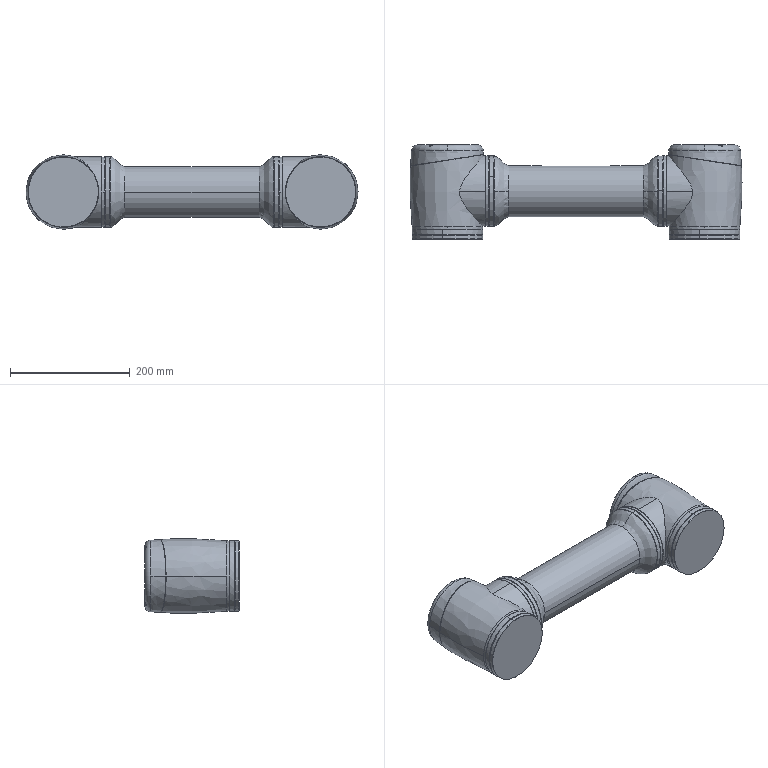Part | SolidWorks | features BaseBody 3 | 3 solids | 505 faces | box 555.047 x 157.65 x 125.047 mm | volume 5841153 mm3 | plane 323 | spline 100 | cylinder 54 | torus 20 | cone 8 | commonest cylinder face diameters 118 x32 6.2 x12 3.5 x2 53.612 x2 85 x2 116.977 x2